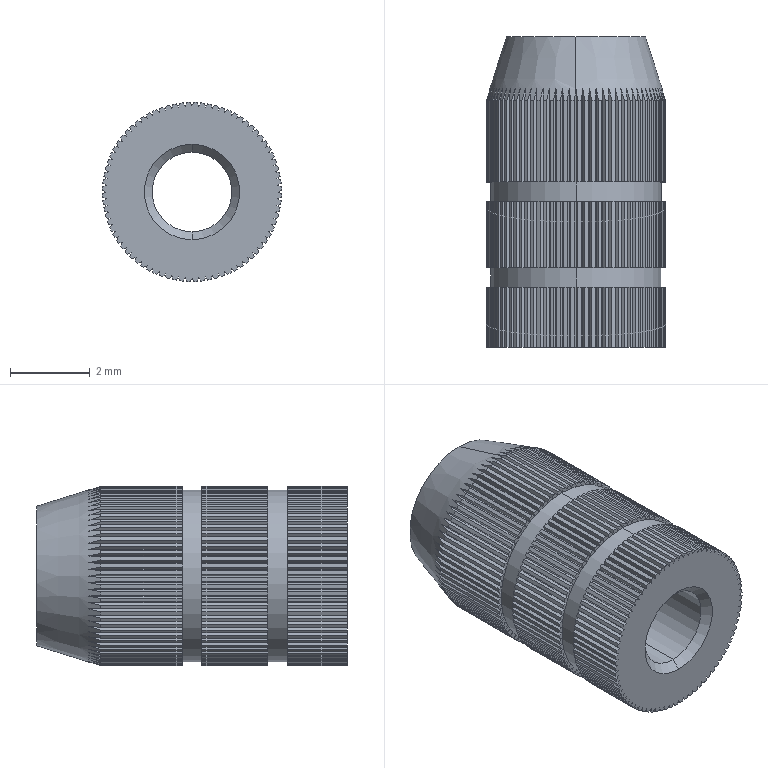Part | SolidWorks | features CirPattern 1, ICE 1, RevCut 1, Revolution 1 | 1 solid | 736 faces | box 4.499 x 7.8 x 4.499 mm | volume 91.087 mm3 | plane 486 | cylinder 246 | cone 4 | commonest cylinder face diameters 4.5 x240 4.3 x4 2 x2